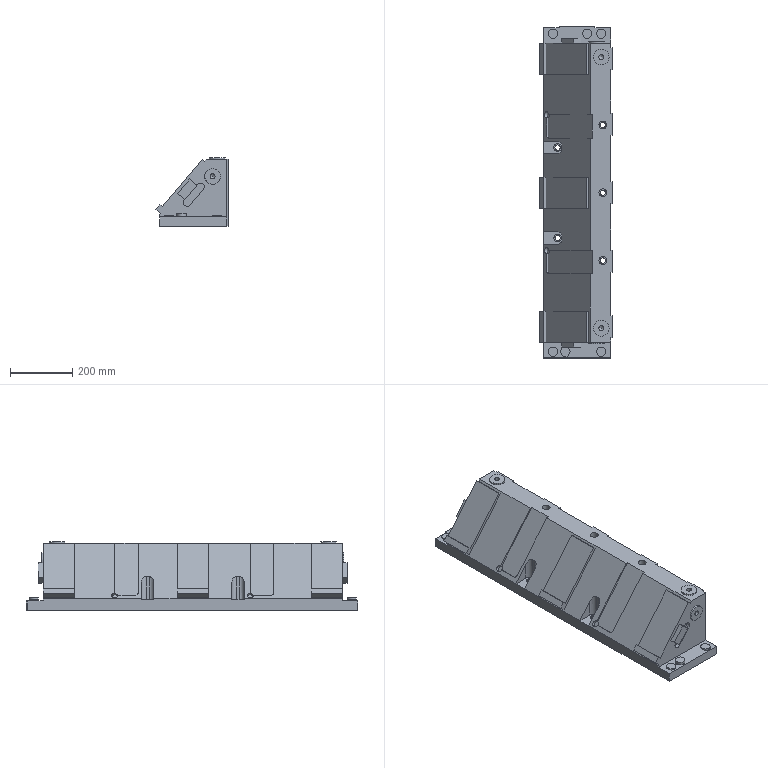Part | NX | features solid 2 | 1 solid | 165 faces | box 231.869 x 1065 x 220 mm | volume 24062526 mm3 | plane 125 | cylinder 36 | cone 4 | commonest cylinder face diameters 30 x10 25 x9 17 x5 16 x4 20 x4 50 x4